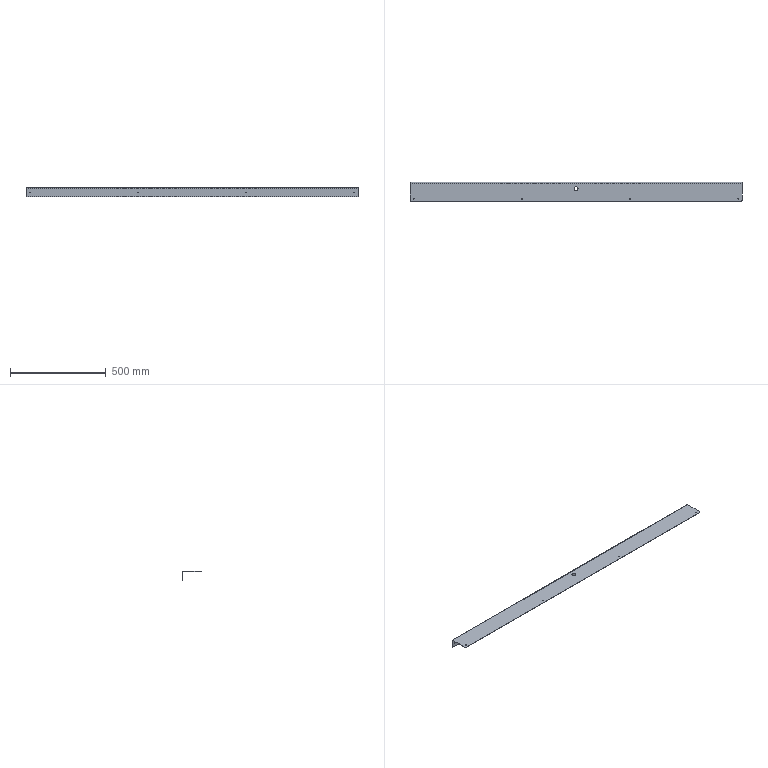Part | NX | features BREP 1 | 1 solid | 34 faces | box 1730 x 99.289 x 48.489 mm | volume 374057 mm3 | cylinder 22 | plane 12 | commonest cylinder face diameters 4.953 x16 12.7 x2 20.65 x2 6.35 x1 9.347 x1
STEP:
#1=CARTESIAN_POINT('',(1729.74,6.35,0.));
#2=VERTEX_POINT('',#1);
#3=CARTESIAN_POINT('',(1729.74,94.615,0.));
#4=VERTEX_POINT('',#3);
#5=CARTESIAN_POINT('',(1729.74,6.35,0.));
#6=DIRECTION('',(0.,1.,0.));
#7=VECTOR('',#6,1000.);
#8=LINE('',#5,#7);
#9=EDGE_CURVE('',#2,#4,#8,.T.);
#10=ORIENTED_EDGE('',*,*,#9,.T.);
#11=CARTESIAN_POINT('',(0.,94.615,0.));
#12=VERTEX_POINT('',#11);
#13=CARTESIAN_POINT('',(0.,94.615,0.));
#14=DIRECTION('',(1.,0.,0.));
#15=VECTOR('',#14,1000.);
#16=LINE('',#13,#15);
#17=EDGE_CURVE('',#12,#4,#16,.T.);
#18=ORIENTED_EDGE('',*,*,#17,.F.);
#19=CARTESIAN_POINT('',(0.,6.35,0.));
#20=VERTEX_POINT('',#19);
#21=CARTESIAN_POINT('',(0.,94.615,0.));
#22=DIRECTION('',(0.,-1.,0.));
#23=VECTOR('',#22,1000.);
#24=LINE('',#21,#23);
#25=EDGE_CURVE('',#12,#20,#24,.T.);
#26=ORIENTED_EDGE('',*,*,#25,.T.);
#27=CARTESIAN_POINT('',(6.35,0.,0.));
#28=VERTEX_POINT('',#27);
#29=CARTESIAN_POINT('',(6.35,6.35,0.));
#30=DIRECTION('',(0.,0.,1.));
#31=DIRECTION('',(-1.,0.,0.));
#32=AXIS2_PLACEMENT_3D('',#29,#30,#31);
#33=CIRCLE('',#32,6.35);
#34=EDGE_CURVE('',#20,#28,#33,.T.);
#35=ORIENTED_EDGE('',*,*,#34,.T.);
#36=CARTESIAN_POINT('',(1723.39,0.,0.));
#37=VERTEX_POINT('',#36);
#38=CARTESIAN_POINT('',(6.35,0.,0.));
#39=DIRECTION('',(1.,0.,0.));
#40=VECTOR('',#39,1000.);
#41=LINE('',#38,#40);
#42=EDGE_CURVE('',#28,#37,#41,.T.);
#43=ORIENTED_EDGE('',*,*,#42,.T.);
#44=CARTESIAN_POINT('',(1723.39,6.35,0.));
#45=DIRECTION('',(0.,0.,1.));
#46=DIRECTION('',(0.,-1.,0.));
#47=AXIS2_PLACEMENT_3D('',#44,#45,#46);
#48=CIRCLE('',#47,6.35);
#49=EDGE_CURVE('',#37,#2,#48,.T.);
#50=ORIENTED_EDGE('',*,*,#49,.T.);
#51=EDGE_LOOP('',(#10,#18,#26,#35,#43,#50));
#52=FACE_BOUND('',#51,.T.);
#53=CARTESIAN_POINT('',(21.526,15.24,0.));
#54=VERTEX_POINT('',#53);
#55=CARTESIAN_POINT('',(16.573,15.24,0.));
#56=VERTEX_POINT('',#55);
#57=CARTESIAN_POINT('',(19.05,15.24,0.));
#58=DIRECTION('',(0.,0.,1.));
#59=DIRECTION('',(1.,0.,0.));
#60=AXIS2_PLACEMENT_3D('',#57,#58,#59);
#61=CIRCLE('',#60,2.477);
#62=EDGE_CURVE('',#54,#56,#61,.T.);
#63=ORIENTED_EDGE('',*,*,#62,.F.);
#64=CARTESIAN_POINT('',(19.05,15.24,0.));
#65=DIRECTION('',(0.,0.,1.));
#66=DIRECTION('',(-1.,0.,0.));
#67=AXIS2_PLACEMENT_3D('',#64,#65,#66);
#68=CIRCLE('',#67,2.477);
#69=EDGE_CURVE('',#56,#54,#68,.T.);
#70=ORIENTED_EDGE('',*,*,#69,.F.);
#71=EDGE_LOOP('',(#63,#70));
#72=FACE_BOUND('',#71,.T.);
#73=CARTESIAN_POINT('',(585.407,15.24,0.));
#74=VERTEX_POINT('',#73);
#75=CARTESIAN_POINT('',(580.453,15.24,0.));
#76=VERTEX_POINT('',#75);
#77=CARTESIAN_POINT('',(582.93,15.24,0.));
#78=DIRECTION('',(0.,0.,1.));
#79=DIRECTION('',(1.,0.,0.));
#80=AXIS2_PLACEMENT_3D('',#77,#78,#79);
#81=CIRCLE('',#80,2.476);
#82=EDGE_CURVE('',#74,#76,#81,.T.);
#83=ORIENTED_EDGE('',*,*,#82,.F.);
#84=CARTESIAN_POINT('',(582.93,15.24,0.));
#85=DIRECTION('',(0.,0.,1.));
#86=DIRECTION('',(-1.,0.,0.));
#87=AXIS2_PLACEMENT_3D('',#84,#85,#86);
#88=CIRCLE('',#87,2.476);
#89=EDGE_CURVE('',#76,#74,#88,.T.);
#90=ORIENTED_EDGE('',*,*,#89,.F.);
#91=EDGE_LOOP('',(#83,#90));
#92=FACE_BOUND('',#91,.T.);
#93=CARTESIAN_POINT('',(1149.286,15.24,0.));
#94=VERTEX_POINT('',#93);
#95=CARTESIAN_POINT('',(1144.333,15.24,0.));
#96=VERTEX_POINT('',#95);
#97=CARTESIAN_POINT('',(1146.81,15.24,0.));
#98=DIRECTION('',(0.,0.,1.));
#99=DIRECTION('',(1.,0.,0.));
#100=AXIS2_PLACEMENT_3D('',#97,#98,#99);
#101=CIRCLE('',#100,2.476);
#102=EDGE_CURVE('',#94,#96,#101,.T.);
#103=ORIENTED_EDGE('',*,*,#102,.F.);
#104=CARTESIAN_POINT('',(1146.81,15.24,0.));
#105=DIRECTION('',(0.,0.,1.));
#106=DIRECTION('',(-1.,0.,0.));
#107=AXIS2_PLACEMENT_3D('',#104,#105,#106);
#108=CIRCLE('',#107,2.476);
#109=EDGE_CURVE('',#96,#94,#108,.T.);
#110=ORIENTED_EDGE('',*,*,#109,.F.);
#111=EDGE_LOOP('',(#103,#110));
#112=FACE_BOUND('',#111,.T.);
#113=CARTESIAN_POINT('',(1713.167,15.24,0.));
#114=VERTEX_POINT('',#113);
#115=CARTESIAN_POINT('',(1708.214,15.24,0.));
#116=VERTEX_POINT('',#115);
#117=CARTESIAN_POINT('',(1710.69,15.24,0.));
#118=DIRECTION('',(0.,0.,1.));
#119=DIRECTION('',(1.,0.,0.));
#120=AXIS2_PLACEMENT_3D('',#117,#118,#119);
#121=CIRCLE('',#120,2.476);
#122=EDGE_CURVE('',#114,#116,#121,.T.);
#123=ORIENTED_EDGE('',*,*,#122,.F.);
#124=CARTESIAN_POINT('',(1710.69,15.24,0.));
#125=DIRECTION('',(0.,0.,1.));
#126=DIRECTION('',(-1.,0.,0.));
#127=AXIS2_PLACEMENT_3D('',#124,#125,#126);
#128=CIRCLE('',#127,2.476);
#129=EDGE_CURVE('',#116,#114,#128,.T.);
#130=ORIENTED_EDGE('',*,*,#129,.F.);
#131=EDGE_LOOP('',(#123,#130));
#132=FACE_BOUND('',#131,.T.);
#133=CARTESIAN_POINT('',(875.322,66.802,0.));
#134=VERTEX_POINT('',#133);
#135=CARTESIAN_POINT('',(854.672,66.802,0.));
#136=VERTEX_POINT('',#135);
#137=CARTESIAN_POINT('',(864.997,66.802,0.));
#138=DIRECTION('',(0.,0.,1.));
#139=DIRECTION('',(1.,0.,0.));
#140=AXIS2_PLACEMENT_3D('',#137,#138,#139);
#141=CIRCLE('',#140,10.325);
#142=EDGE_CURVE('',#134,#136,#141,.T.);
#143=ORIENTED_EDGE('',*,*,#142,.F.);
#144=CARTESIAN_POINT('',(864.997,66.802,0.));
#145=DIRECTION('',(0.,0.,1.));
#146=DIRECTION('',(-1.,0.,0.));
#147=AXIS2_PLACEMENT_3D('',#144,#145,#146);
#148=CIRCLE('',#147,10.325);
#149=EDGE_CURVE('',#136,#134,#148,.T.);
#150=ORIENTED_EDGE('',*,*,#149,.F.);
#151=EDGE_LOOP('',(#143,#150));
#152=FACE_BOUND('',#151,.T.);
#153=CARTESIAN_POINT('',(0.,0.,0.));
#154=DIRECTION('',(0.,0.,1.));
#155=DIRECTION('',(1.,0.,0.));
#156=AXIS2_PLACEMENT_3D('',#153,#154,#155);
#157=PLANE('',#156);
#158=ADVANCED_FACE('',(#52,#72,#92,#112,#132,#152),#157,.T.);
#159=CARTESIAN_POINT('',(1729.74,6.35,-1.499));
#160=VERTEX_POINT('',#159);
#161=CARTESIAN_POINT('',(1723.39,0.,-1.499));
#162=VERTEX_POINT('',#161);
#163=CARTESIAN_POINT('',(1723.39,6.35,-1.499));
#164=DIRECTION('',(0.,0.,-1.));
#165=DIRECTION('',(1.,0.,0.));
#166=AXIS2_PLACEMENT_3D('',#163,#164,#165);
#167=CIRCLE('',#166,6.35);
#168=EDGE_CURVE('',#160,#162,#167,.T.);
#169=ORIENTED_EDGE('',*,*,#168,.F.);
#170=CARTESIAN_POINT('',(1729.74,6.35,-1.499));
#171=DIRECTION('',(0.,0.,1.));
#172=VECTOR('',#171,1000.);
#173=LINE('',#170,#172);
#174=EDGE_CURVE('',#160,#2,#173,.T.);
#175=ORIENTED_EDGE('',*,*,#174,.T.);
#176=ORIENTED_EDGE('',*,*,#49,.F.);
#177=CARTESIAN_POINT('',(1723.39,0.,-1.499));
#178=DIRECTION('',(0.,0.,1.));
#179=VECTOR('',#178,1000.);
#180=LINE('',#177,#179);
#181=EDGE_CURVE('',#162,#37,#180,.T.);
#182=ORIENTED_EDGE('',*,*,#181,.F.);
#183=EDGE_LOOP('',(#169,#175,#176,#182));
#184=FACE_BOUND('',#183,.T.);
#185=CARTESIAN_POINT('',(1723.39,6.35,-3.816));
#186=DIRECTION('',(0.,0.,1.));
#187=DIRECTION('',(0.,-1.,0.));
#188=AXIS2_PLACEMENT_3D('',#185,#186,#187);
#189=CYLINDRICAL_SURFACE('',#188,6.35);
#190=ADVANCED_FACE('',(#184),#189,.T.);
#191=ORIENTED_EDGE('',*,*,#42,.F.);
#192=CARTESIAN_POINT('',(6.35,0.,-1.499));
#193=VERTEX_POINT('',#192);
#194=CARTESIAN_POINT('',(6.35,0.,-1.499));
#195=DIRECTION('',(0.,0.,1.));
#196=VECTOR('',#195,1000.);
#197=LINE('',#194,#196);
#198=EDGE_CURVE('',#193,#28,#197,.T.);
#199=ORIENTED_EDGE('',*,*,#198,.F.);
#200=CARTESIAN_POINT('',(6.35,0.,-1.499));
#201=DIRECTION('',(1.,0.,0.));
#202=VECTOR('',#201,1000.);
#203=LINE('',#200,#202);
#204=EDGE_CURVE('',#193,#162,#203,.T.);
#205=ORIENTED_EDGE('',*,*,#204,.T.);
#206=ORIENTED_EDGE('',*,*,#181,.T.);
#207=EDGE_LOOP('',(#191,#199,#205,#206));
#208=FACE_BOUND('',#207,.T.);
#209=CARTESIAN_POINT('',(864.87,0.,-0.7493));
#210=DIRECTION('',(0.,-1.,0.));
#211=DIRECTION('',(0.,0.,-1.));
#212=AXIS2_PLACEMENT_3D('',#209,#210,#211);
#213=PLANE('',#212);
#214=ADVANCED_FACE('',(#208),#213,.T.);
#215=ORIENTED_EDGE('',*,*,#204,.F.);
#216=CARTESIAN_POINT('',(0.,6.35,-1.499));
#217=VERTEX_POINT('',#216);
#218=CARTESIAN_POINT('',(6.35,6.35,-1.499));
#219=DIRECTION('',(0.,0.,-1.));
#220=DIRECTION('',(0.,-1.,0.));
#221=AXIS2_PLACEMENT_3D('',#218,#219,#220);
#222=CIRCLE('',#221,6.35);
#223=EDGE_CURVE('',#193,#217,#222,.T.);
#224=ORIENTED_EDGE('',*,*,#223,.T.);
#225=CARTESIAN_POINT('',(0.,94.615,-1.499));
#226=VERTEX_POINT('',#225);
#227=CARTESIAN_POINT('',(0.,94.615,-1.499));
#228=DIRECTION('',(0.,-1.,0.));
#229=VECTOR('',#228,1000.);
#230=LINE('',#227,#229);
#231=EDGE_CURVE('',#226,#217,#230,.T.);
#232=ORIENTED_EDGE('',*,*,#231,.F.);
#233=CARTESIAN_POINT('',(1729.74,94.615,-1.499));
#234=VERTEX_POINT('',#233);
#235=CARTESIAN_POINT('',(0.,94.615,-1.499));
#236=DIRECTION('',(1.,0.,0.));
#237=VECTOR('',#236,1000.);
#238=LINE('',#235,#237);
#239=EDGE_CURVE('',#226,#234,#238,.T.);
#240=ORIENTED_EDGE('',*,*,#239,.T.);
#241=CARTESIAN_POINT('',(1729.74,6.35,-1.499));
#242=DIRECTION('',(0.,1.,0.));
#243=VECTOR('',#242,1000.);
#244=LINE('',#241,#243);
#245=EDGE_CURVE('',#160,#234,#244,.T.);
#246=ORIENTED_EDGE('',*,*,#245,.F.);
#247=ORIENTED_EDGE('',*,*,#168,.T.);
#248=EDGE_LOOP('',(#215,#224,#232,#240,#246,#247));
#249=FACE_BOUND('',#248,.T.);
#250=CARTESIAN_POINT('',(21.526,15.24,-1.499));
#251=VERTEX_POINT('',#250);
#252=CARTESIAN_POINT('',(16.573,15.24,-1.499));
#253=VERTEX_POINT('',#252);
#254=CARTESIAN_POINT('',(19.05,15.24,-1.499));
#255=DIRECTION('',(0.,0.,1.));
#256=DIRECTION('',(1.,0.,0.));
#257=AXIS2_PLACEMENT_3D('',#254,#255,#256);
#258=CIRCLE('',#257,2.477);
#259=EDGE_CURVE('',#251,#253,#258,.T.);
#260=ORIENTED_EDGE('',*,*,#259,.T.);
#261=CARTESIAN_POINT('',(19.05,15.24,-1.499));
#262=DIRECTION('',(0.,0.,1.));
#263=DIRECTION('',(-1.,0.,0.));
#264=AXIS2_PLACEMENT_3D('',#261,#262,#263);
#265=CIRCLE('',#264,2.477);
#266=EDGE_CURVE('',#253,#251,#265,.T.);
#267=ORIENTED_EDGE('',*,*,#266,.T.);
#268=EDGE_LOOP('',(#260,#267));
#269=FACE_BOUND('',#268,.T.);
#270=CARTESIAN_POINT('',(585.407,15.24,-1.499));
#271=VERTEX_POINT('',#270);
#272=CARTESIAN_POINT('',(580.453,15.24,-1.499));
#273=VERTEX_POINT('',#272);
#274=CARTESIAN_POINT('',(582.93,15.24,-1.499));
#275=DIRECTION('',(0.,0.,1.));
#276=DIRECTION('',(1.,0.,0.));
#277=AXIS2_PLACEMENT_3D('',#274,#275,#276);
#278=CIRCLE('',#277,2.476);
#279=EDGE_CURVE('',#271,#273,#278,.T.);
#280=ORIENTED_EDGE('',*,*,#279,.T.);
#281=CARTESIAN_POINT('',(582.93,15.24,-1.499));
#282=DIRECTION('',(0.,0.,1.));
#283=DIRECTION('',(-1.,0.,0.));
#284=AXIS2_PLACEMENT_3D('',#281,#282,#283);
#285=CIRCLE('',#284,2.476);
#286=EDGE_CURVE('',#273,#271,#285,.T.);
#287=ORIENTED_EDGE('',*,*,#286,.T.);
#288=EDGE_LOOP('',(#280,#287));
#289=FACE_BOUND('',#288,.T.);
#290=CARTESIAN_POINT('',(1149.286,15.24,-1.499));
#291=VERTEX_POINT('',#290);
#292=CARTESIAN_POINT('',(1144.333,15.24,-1.499));
#293=VERTEX_POINT('',#292);
#294=CARTESIAN_POINT('',(1146.81,15.24,-1.499));
#295=DIRECTION('',(0.,0.,1.));
#296=DIRECTION('',(1.,0.,0.));
#297=AXIS2_PLACEMENT_3D('',#294,#295,#296);
#298=CIRCLE('',#297,2.476);
#299=EDGE_CURVE('',#291,#293,#298,.T.);
#300=ORIENTED_EDGE('',*,*,#299,.T.);
#301=CARTESIAN_POINT('',(1146.81,15.24,-1.499));
#302=DIRECTION('',(0.,0.,1.));
#303=DIRECTION('',(-1.,0.,0.));
#304=AXIS2_PLACEMENT_3D('',#301,#302,#303);
#305=CIRCLE('',#304,2.476);
#306=EDGE_CURVE('',#293,#291,#305,.T.);
#307=ORIENTED_EDGE('',*,*,#306,.T.);
#308=EDGE_LOOP('',(#300,#307));
#309=FACE_BOUND('',#308,.T.);
#310=CARTESIAN_POINT('',(1713.167,15.24,-1.499));
#311=VERTEX_POINT('',#310);
#312=CARTESIAN_POINT('',(1708.214,15.24,-1.499));
#313=VERTEX_POINT('',#312);
#314=CARTESIAN_POINT('',(1710.69,15.24,-1.499));
#315=DIRECTION('',(0.,0.,1.));
#316=DIRECTION('',(1.,0.,0.));
#317=AXIS2_PLACEMENT_3D('',#314,#315,#316);
#318=CIRCLE('',#317,2.476);
#319=EDGE_CURVE('',#311,#313,#318,.T.);
#320=ORIENTED_EDGE('',*,*,#319,.T.);
#321=CARTESIAN_POINT('',(1710.69,15.24,-1.499));
#322=DIRECTION('',(0.,0.,1.));
#323=DIRECTION('',(-1.,0.,0.));
#324=AXIS2_PLACEMENT_3D('',#321,#322,#323);
#325=CIRCLE('',#324,2.476);
#326=EDGE_CURVE('',#313,#311,#325,.T.);
#327=ORIENTED_EDGE('',*,*,#326,.T.);
#328=EDGE_LOOP('',(#320,#327));
#329=FACE_BOUND('',#328,.T.);
#330=CARTESIAN_POINT('',(875.322,66.802,-1.499));
#331=VERTEX_POINT('',#330);
#332=CARTESIAN_POINT('',(854.672,66.802,-1.499));
#333=VERTEX_POINT('',#332);
#334=CARTESIAN_POINT('',(864.997,66.802,-1.499));
#335=DIRECTION('',(0.,0.,1.));
#336=DIRECTION('',(1.,0.,0.));
#337=AXIS2_PLACEMENT_3D('',#334,#335,#336);
#338=CIRCLE('',#337,10.325);
#339=EDGE_CURVE('',#331,#333,#338,.T.);
#340=ORIENTED_EDGE('',*,*,#339,.T.);
#341=CARTESIAN_POINT('',(864.997,66.802,-1.499));
#342=DIRECTION('',(0.,0.,1.));
#343=DIRECTION('',(-1.,0.,0.));
#344=AXIS2_PLACEMENT_3D('',#341,#342,#343);
#345=CIRCLE('',#344,10.325);
#346=EDGE_CURVE('',#333,#331,#345,.T.);
#347=ORIENTED_EDGE('',*,*,#346,.T.);
#348=EDGE_LOOP('',(#340,#347));
#349=FACE_BOUND('',#348,.T.);
#350=CARTESIAN_POINT('',(0.,0.,-1.499));
#351=DIRECTION('',(0.,0.,1.));
#352=DIRECTION('',(1.,0.,0.));
#353=AXIS2_PLACEMENT_3D('',#350,#351,#352);
#354=PLANE('',#353);
#355=ADVANCED_FACE('',(#249,#269,#289,#309,#329,#349),#354,.F.);
#356=ORIENTED_EDGE('',*,*,#245,.T.);
#357=CARTESIAN_POINT('',(1729.74,94.615,-1.499));
#358=DIRECTION('',(0.,0.,1.));
#359=VECTOR('',#358,1000.);
#360=LINE('',#357,#359);
#361=EDGE_CURVE('',#234,#4,#360,.T.);
#362=ORIENTED_EDGE('',*,*,#361,.T.);
#363=ORIENTED_EDGE('',*,*,#9,.F.);
#364=ORIENTED_EDGE('',*,*,#174,.F.);
#365=EDGE_LOOP('',(#356,#362,#363,#364));
#366=FACE_BOUND('',#365,.T.);
#367=CARTESIAN_POINT('',(1729.74,48.895,-0.7493));
#368=DIRECTION('',(1.,0.,0.));
#369=DIRECTION('',(0.,1.,0.));
#370=AXIS2_PLACEMENT_3D('',#367,#368,#369);
#371=PLANE('',#370);
#372=ADVANCED_FACE('',(#366),#371,.T.);
#373=CARTESIAN_POINT('',(1729.74,97.79,-4.674));
#374=VERTEX_POINT('',#373);
#375=CARTESIAN_POINT('',(1729.74,99.289,-4.674));
#376=VERTEX_POINT('',#375);
#377=CARTESIAN_POINT('',(1729.74,97.79,-4.674));
#378=DIRECTION('',(0.,1.,0.));
#379=VECTOR('',#378,1000.);
#380=LINE('',#377,#379);
#381=EDGE_CURVE('',#374,#376,#380,.T.);
#382=ORIENTED_EDGE('',*,*,#381,.T.);
#383=CARTESIAN_POINT('',(1729.74,94.615,-4.674));
#384=DIRECTION('',(1.,0.,0.));
#385=DIRECTION('',(0.,1.,0.));
#386=AXIS2_PLACEMENT_3D('',#383,#384,#385);
#387=CIRCLE('',#386,4.674);
#388=EDGE_CURVE('',#376,#4,#387,.T.);
#389=ORIENTED_EDGE('',*,*,#388,.T.);
#390=ORIENTED_EDGE('',*,*,#361,.F.);
#391=CARTESIAN_POINT('',(1729.74,94.615,-4.674));
#392=DIRECTION('',(1.,0.,0.));
#393=DIRECTION('',(0.,1.,0.));
#394=AXIS2_PLACEMENT_3D('',#391,#392,#393);
#395=CIRCLE('',#394,3.175);
#396=EDGE_CURVE('',#374,#234,#395,.T.);
#397=ORIENTED_EDGE('',*,*,#396,.F.);
#398=EDGE_LOOP('',(#382,#389,#390,#397));
#399=FACE_BOUND('',#398,.T.);
#400=CARTESIAN_POINT('',(1729.74,97.39,-1.899));
#401=DIRECTION('',(1.,0.,0.));
#402=DIRECTION('',(0.,1.,0.));
#403=AXIS2_PLACEMENT_3D('',#400,#401,#402);
#404=PLANE('',#403);
#405=ADVANCED_FACE('',(#399),#404,.T.);
#406=ORIENTED_EDGE('',*,*,#396,.T.);
#407=ORIENTED_EDGE('',*,*,#239,.F.);
#408=CARTESIAN_POINT('',(0.,97.79,-4.674));
#409=VERTEX_POINT('',#408);
#410=CARTESIAN_POINT('',(0.,94.615,-4.674));
#411=DIRECTION('',(1.,0.,0.));
#412=DIRECTION('',(0.,1.,0.));
#413=AXIS2_PLACEMENT_3D('',#410,#411,#412);
#414=CIRCLE('',#413,3.175);
#415=EDGE_CURVE('',#409,#226,#414,.T.);
#416=ORIENTED_EDGE('',*,*,#415,.F.);
#417=CARTESIAN_POINT('',(0.,97.79,-4.674));
#418=DIRECTION('',(1.,0.,0.));
#419=VECTOR('',#418,1000.);
#420=LINE('',#417,#419);
#421=EDGE_CURVE('',#409,#374,#420,.T.);
#422=ORIENTED_EDGE('',*,*,#421,.T.);
#423=EDGE_LOOP('',(#406,#407,#416,#422));
#424=FACE_BOUND('',#423,.T.);
#425=CARTESIAN_POINT('',(0.,94.615,-4.674));
#426=DIRECTION('',(1.,0.,0.));
#427=DIRECTION('',(0.,1.,0.));
#428=AXIS2_PLACEMENT_3D('',#425,#426,#427);
#429=CYLINDRICAL_SURFACE('',#428,3.175);
#430=ADVANCED_FACE('',(#424),#429,.F.);
#431=ORIENTED_EDGE('',*,*,#421,.F.);
#432=CARTESIAN_POINT('',(0.,97.79,-48.489));
#433=VERTEX_POINT('',#432);
#434=CARTESIAN_POINT('',(0.,97.79,-48.489));
#435=DIRECTION('',(0.,0.,1.));
#436=VECTOR('',#435,1000.);
#437=LINE('',#434,#436);
#438=EDGE_CURVE('',#433,#409,#437,.T.);
#439=ORIENTED_EDGE('',*,*,#438,.F.);
#440=CARTESIAN_POINT('',(1729.74,97.79,-48.489));
#441=VERTEX_POINT('',#440);
#442=CARTESIAN_POINT('',(1729.74,97.79,-48.489));
#443=DIRECTION('',(-1.,0.,0.));
#444=VECTOR('',#443,1000.);
#445=LINE('',#442,#444);
#446=EDGE_CURVE('',#441,#433,#445,.T.);
#447=ORIENTED_EDGE('',*,*,#446,.F.);
#448=CARTESIAN_POINT('',(1729.74,97.79,-4.674));
#449=DIRECTION('',(0.,0.,-1.));
#450=VECTOR('',#449,1000.);
#451=LINE('',#448,#450);
#452=EDGE_CURVE('',#374,#441,#451,.T.);
#453=ORIENTED_EDGE('',*,*,#452,.F.);
#454=EDGE_LOOP('',(#431,#439,#447,#453));
#455=FACE_BOUND('',#454,.T.);
#456=CARTESIAN_POINT('',(21.526,97.79,-26.899));
#457=VERTEX_POINT('',#456);
#458=CARTESIAN_POINT('',(16.573,97.79,-26.899));
#459=VERTEX_POINT('',#458);
#460=CARTESIAN_POINT('',(19.05,97.79,-26.899));
#461=DIRECTION('',(0.,1.,0.));
#462=DIRECTION('',(1.,0.,0.));
#463=AXIS2_PLACEMENT_3D('',#460,#461,#462);
#464=CIRCLE('',#463,2.477);
#465=EDGE_CURVE('',#457,#459,#464,.T.);
#466=ORIENTED_EDGE('',*,*,#465,.T.);
#467=CARTESIAN_POINT('',(19.05,97.79,-26.899));
#468=DIRECTION('',(0.,1.,0.));
#469=DIRECTION('',(-1.,0.,0.));
#470=AXIS2_PLACEMENT_3D('',#467,#468,#469);
#471=CIRCLE('',#470,2.477);
#472=EDGE_CURVE('',#459,#457,#471,.T.);
#473=ORIENTED_EDGE('',*,*,#472,.T.);
#474=EDGE_LOOP('',(#466,#473));
#475=FACE_BOUND('',#474,.T.);
#476=CARTESIAN_POINT('',(585.407,97.79,-26.899));
#477=VERTEX_POINT('',#476);
#478=CARTESIAN_POINT('',(580.453,97.79,-26.899));
#479=VERTEX_POINT('',#478);
#480=CARTESIAN_POINT('',(582.93,97.79,-26.899));
#481=DIRECTION('',(0.,1.,0.));
#482=DIRECTION('',(1.,0.,0.));
#483=AXIS2_PLACEMENT_3D('',#480,#481,#482);
#484=CIRCLE('',#483,2.476);
#485=EDGE_CURVE('',#477,#479,#484,.T.);
#486=ORIENTED_EDGE('',*,*,#485,.T.);
#487=CARTESIAN_POINT('',(582.93,97.79,-26.899));
#488=DIRECTION('',(0.,1.,0.));
#489=DIRECTION('',(-1.,0.,0.));
#490=AXIS2_PLACEMENT_3D('',#487,#488,#489);
#491=CIRCLE('',#490,2.476);
#492=EDGE_CURVE('',#479,#477,#491,.T.);
#493=ORIENTED_EDGE('',*,*,#492,.T.);
#494=EDGE_LOOP('',(#486,#493));
#495=FACE_BOUND('',#494,.T.);
#496=CARTESIAN_POINT('',(1149.286,97.79,-26.899));
#497=VERTEX_POINT('',#496);
#498=CARTESIAN_POINT('',(1144.333,97.79,-26.899));
#499=VERTEX_POINT('',#498);
#500=CARTESIAN_POINT('',(1146.81,97.79,-26.899));
#501=DIRECTION('',(0.,1.,0.));
#502=DIRECTION('',(1.,0.,0.));
#503=AXIS2_PLACEMENT_3D('',#500,#501,#502);
#504=CIRCLE('',#503,2.476);
#505=EDGE_CURVE('',#497,#499,#504,.T.);
#506=ORIENTED_EDGE('',*,*,#505,.T.);
#507=CARTESIAN_POINT('',(1146.81,97.79,-26.899));
#508=DIRECTION('',(0.,1.,0.));
#509=DIRECTION('',(-1.,0.,0.));
#510=AXIS2_PLACEMENT_3D('',#507,#508,#509);
#511=CIRCLE('',#510,2.476);
#512=EDGE_CURVE('',#499,#497,#511,.T.);
#513=ORIENTED_EDGE('',*,*,#512,.T.);
#514=EDGE_LOOP('',(#506,#513));
#515=FACE_BOUND('',#514,.T.);
#516=CARTESIAN_POINT('',(1713.167,97.79,-26.899));
#517=VERTEX_POINT('',#516);
#518=CARTESIAN_POINT('',(1708.214,97.79,-26.899));
#519=VERTEX_POINT('',#518);
#520=CARTESIAN_POINT('',(1710.69,97.79,-26.899));
#521=DIRECTION('',(0.,1.,0.));
#522=DIRECTION('',(1.,0.,0.));
#523=AXIS2_PLACEMENT_3D('',#520,#521,#522);
#524=CIRCLE('',#523,2.476);
#525=EDGE_CURVE('',#517,#519,#524,.T.);
#526=ORIENTED_EDGE('',*,*,#525,.T.);
#527=CARTESIAN_POINT('',(1710.69,97.79,-26.899));
#528=DIRECTION('',(0.,1.,0.));
#529=DIRECTION('',(-1.,0.,0.));
#530=AXIS2_PLACEMENT_3D('',#527,#528,#529);
#531=CIRCLE('',#530,2.476);
#532=EDGE_CURVE('',#519,#517,#531,.T.);
#533=ORIENTED_EDGE('',*,*,#532,.T.);
#534=EDGE_LOOP('',(#526,#533));
#535=FACE_BOUND('',#534,.T.);
#536=CARTESIAN_POINT('',(1318.754,97.79,-1.499));
#537=DIRECTION('',(0.,1.,0.));
#538=DIRECTION('',(1.,0.,0.));
#539=AXIS2_PLACEMENT_3D('',#536,#537,#538);
#540=PLANE('',#539);
#541=ADVANCED_FACE('',(#455,#475,#495,#515,#535),#540,.F.);
#542=CARTESIAN_POINT('',(1729.74,99.289,-48.489));
#543=VERTEX_POINT('',#542);
#544=CARTESIAN_POINT('',(1729.74,97.79,-48.489));
#545=DIRECTION('',(0.,1.,0.));
#546=VECTOR('',#545,1000.);
#547=LINE('',#544,#546);
#548=EDGE_CURVE('',#441,#543,#547,.T.);
#549=ORIENTED_EDGE('',*,*,#548,.T.);
#550=CARTESIAN_POINT('',(1729.74,99.289,-4.674));
#551=DIRECTION('',(0.,0.,-1.));
#552=VECTOR('',#551,1000.);
#553=LINE('',#550,#552);
#554=EDGE_CURVE('',#376,#543,#553,.T.);
#555=ORIENTED_EDGE('',*,*,#554,.F.);
#556=ORIENTED_EDGE('',*,*,#381,.F.);
#557=ORIENTED_EDGE('',*,*,#452,.T.);
#558=EDGE_LOOP('',(#549,#555,#556,#557));
#559=FACE_BOUND('',#558,.T.);
#560=CARTESIAN_POINT('',(1729.74,98.539,-26.581));
#561=DIRECTION('',(-1.,0.,0.));
#562=DIRECTION('',(0.,0.,1.));
#563=AXIS2_PLACEMENT_3D('',#560,#561,#562);
#564=PLANE('',#563);
#565=ADVANCED_FACE('',(#559),#564,.F.);
#566=CARTESIAN_POINT('',(0.,99.289,-48.489));
#567=VERTEX_POINT('',#566);
#568=CARTESIAN_POINT('',(1729.74,99.289,-48.489));
#569=DIRECTION('',(-1.,0.,0.));
#570=VECTOR('',#569,1000.);
#571=LINE('',#568,#570);
#572=EDGE_CURVE('',#543,#567,#571,.T.);
#573=ORIENTED_EDGE('',*,*,#572,.T.);
#574=CARTESIAN_POINT('',(0.,99.289,-4.674));
#575=VERTEX_POINT('',#574);
#576=CARTESIAN_POINT('',(0.,99.289,-48.489));
#577=DIRECTION('',(0.,0.,1.));
#578=VECTOR('',#577,1000.);
#579=LINE('',#576,#578);
#580=EDGE_CURVE('',#567,#575,#579,.T.);
#581=ORIENTED_EDGE('',*,*,#580,.T.);
#582=CARTESIAN_POINT('',(0.,99.289,-4.674));
#583=DIRECTION('',(1.,0.,0.));
#584=VECTOR('',#583,1000.);
#585=LINE('',#582,#584);
#586=EDGE_CURVE('',#575,#376,#585,.T.);
#587=ORIENTED_EDGE('',*,*,#586,.T.);
#588=ORIENTED_EDGE('',*,*,#554,.T.);
#589=EDGE_LOOP('',(#573,#581,#587,#588));
#590=FACE_BOUND('',#589,.T.);
#591=CARTESIAN_POINT('',(21.526,99.289,-26.899));
#592=VERTEX_POINT('',#591);
#593=CARTESIAN_POINT('',(16.573,99.289,-26.899));
#594=VERTEX_POINT('',#593);
#595=CARTESIAN_POINT('',(19.05,99.289,-26.899));
#596=DIRECTION('',(0.,1.,0.));
#597=DIRECTION('',(1.,0.,0.));
#598=AXIS2_PLACEMENT_3D('',#595,#596,#597);
#599=CIRCLE('',#598,2.477);
#600=EDGE_CURVE('',#592,#594,#599,.T.);
#601=ORIENTED_EDGE('',*,*,#600,.F.);
#602=CARTESIAN_POINT('',(19.05,99.289,-26.899));
#603=DIRECTION('',(0.,1.,0.));
#604=DIRECTION('',(-1.,0.,0.));
#605=AXIS2_PLACEMENT_3D('',#602,#603,#604);
#606=CIRCLE('',#605,2.477);
#607=EDGE_CURVE('',#594,#592,#606,.T.);
#608=ORIENTED_EDGE('',*,*,#607,.F.);
#609=EDGE_LOOP('',(#601,#608));
#610=FACE_BOUND('',#609,.T.);
#611=CARTESIAN_POINT('',(585.407,99.289,-26.899));
#612=VERTEX_POINT('',#611);
#613=CARTESIAN_POINT('',(580.453,99.289,-26.899));
#614=VERTEX_POINT('',#613);
#615=CARTESIAN_POINT('',(582.93,99.289,-26.899));
#616=DIRECTION('',(0.,1.,0.));
#617=DIRECTION('',(1.,0.,0.));
#618=AXIS2_PLACEMENT_3D('',#615,#616,#617);
#619=CIRCLE('',#618,2.476);
#620=EDGE_CURVE('',#612,#614,#619,.T.);
#621=ORIENTED_EDGE('',*,*,#620,.F.);
#622=CARTESIAN_POINT('',(582.93,99.289,-26.899));
#623=DIRECTION('',(0.,1.,0.));
#624=DIRECTION('',(-1.,0.,0.));
#625=AXIS2_PLACEMENT_3D('',#622,#623,#624);
#626=CIRCLE('',#625,2.476);
#627=EDGE_CURVE('',#614,#612,#626,.T.);
#628=ORIENTED_EDGE('',*,*,#627,.F.);
#629=EDGE_LOOP('',(#621,#628));
#630=FACE_BOUND('',#629,.T.);
#631=CARTESIAN_POINT('',(1149.286,99.289,-26.899));
#632=VERTEX_POINT('',#631);
#633=CARTESIAN_POINT('',(1144.333,99.289,-26.899));
#634=VERTEX_POINT('',#633);
#635=CARTESIAN_POINT('',(1146.81,99.289,-26.899));
#636=DIRECTION('',(0.,1.,0.));
#637=DIRECTION('',(1.,0.,0.));
#638=AXIS2_PLACEMENT_3D('',#635,#636,#637);
#639=CIRCLE('',#638,2.476);
#640=EDGE_CURVE('',#632,#634,#639,.T.);
#641=ORIENTED_EDGE('',*,*,#640,.F.);
#642=CARTESIAN_POINT('',(1146.81,99.289,-26.899));
#643=DIRECTION('',(0.,1.,0.));
#644=DIRECTION('',(-1.,0.,0.));
#645=AXIS2_PLACEMENT_3D('',#642,#643,#644);
#646=CIRCLE('',#645,2.476);
#647=EDGE_CURVE('',#634,#632,#646,.T.);
#648=ORIENTED_EDGE('',*,*,#647,.F.);
#649=EDGE_LOOP('',(#641,#648));
#650=FACE_BOUND('',#649,.T.);
#651=CARTESIAN_POINT('',(1713.167,99.289,-26.899));
#652=VERTEX_POINT('',#651);
#653=CARTESIAN_POINT('',(1708.214,99.289,-26.899));
#654=VERTEX_POINT('',#653);
#655=CARTESIAN_POINT('',(1710.69,99.289,-26.899));
#656=DIRECTION('',(0.,1.,0.));
#657=DIRECTION('',(1.,0.,0.));
#658=AXIS2_PLACEMENT_3D('',#655,#656,#657);
#659=CIRCLE('',#658,2.476);
#660=EDGE_CURVE('',#652,#654,#659,.T.);
#661=ORIENTED_EDGE('',*,*,#660,.F.);
#662=CARTESIAN_POINT('',(1710.69,99.289,-26.899));
#663=DIRECTION('',(0.,1.,0.));
#664=DIRECTION('',(-1.,0.,0.));
#665=AXIS2_PLACEMENT_3D('',#662,#663,#664);
#666=CIRCLE('',#665,2.476);
#667=EDGE_CURVE('',#654,#652,#666,.T.);
#668=ORIENTED_EDGE('',*,*,#667,.F.);
#669=EDGE_LOOP('',(#661,#668));
#670=FACE_BOUND('',#669,.T.);
#671=CARTESIAN_POINT('',(1318.754,99.289,-1.499));
#672=DIRECTION('',(0.,1.,0.));
#673=DIRECTION('',(1.,0.,0.));
#674=AXIS2_PLACEMENT_3D('',#671,#672,#673);
#675=PLANE('',#674);
#676=ADVANCED_FACE('',(#590,#610,#630,#650,#670),#675,.T.);
#677=CARTESIAN_POINT('',(0.,94.615,-4.674));
#678=DIRECTION('',(1.,0.,0.));
#679=DIRECTION('',(0.,1.,0.));
#680=AXIS2_PLACEMENT_3D('',#677,#678,#679);
#681=CIRCLE('',#680,4.674);
#682=EDGE_CURVE('',#575,#12,#681,.T.);
#683=ORIENTED_EDGE('',*,*,#682,.T.);
#684=ORIENTED_EDGE('',*,*,#17,.T.);
#685=ORIENTED_EDGE('',*,*,#388,.F.);
#686=ORIENTED_EDGE('',*,*,#586,.F.);
#687=EDGE_LOOP('',(#683,#684,#685,#686));
#688=FACE_BOUND('',#687,.T.);
#689=CARTESIAN_POINT('',(0.,94.615,-4.674));
#690=DIRECTION('',(1.,0.,0.));
#691=DIRECTION('',(0.,1.,0.));
#692=AXIS2_PLACEMENT_3D('',#689,#690,#691);
#693=CYLINDRICAL_SURFACE('',#692,4.674);
#694=ADVANCED_FACE('',(#688),#693,.T.);
#695=CARTESIAN_POINT('',(0.,94.615,-1.499));
#696=DIRECTION('',(0.,0.,1.));
#697=VECTOR('',#696,1000.);
#698=LINE('',#695,#697);
#699=EDGE_CURVE('',#226,#12,#698,.T.);
#700=ORIENTED_EDGE('',*,*,#699,.T.);
#701=ORIENTED_EDGE('',*,*,#682,.F.);
#702=CARTESIAN_POINT('',(0.,97.79,-4.674));
#703=DIRECTION('',(0.,1.,0.));
#704=VECTOR('',#703,1000.);
#705=LINE('',#702,#704);
#706=EDGE_CURVE('',#409,#575,#705,.T.);
#707=ORIENTED_EDGE('',*,*,#706,.F.);
#708=ORIENTED_EDGE('',*,*,#415,.T.);
#709=EDGE_LOOP('',(#700,#701,#707,#708));
#710=FACE_BOUND('',#709,.T.);
#711=CARTESIAN_POINT('',(0.,97.39,-1.899));
#712=DIRECTION('',(1.,0.,0.));
#713=DIRECTION('',(0.,1.,0.));
#714=AXIS2_PLACEMENT_3D('',#711,#712,#713);
#715=PLANE('',#714);
#716=ADVANCED_FACE('',(#710),#715,.F.);
#717=ORIENTED_EDGE('',*,*,#706,.T.);
#718=ORIENTED_EDGE('',*,*,#580,.F.);
#719=CARTESIAN_POINT('',(0.,97.79,-48.489));
#720=DIRECTION('',(0.,1.,0.));
#721=VECTOR('',#720,1000.);
#722=LINE('',#719,#721);
#723=EDGE_CURVE('',#433,#567,#722,.T.);
#724=ORIENTED_EDGE('',*,*,#723,.F.);
#725=ORIENTED_EDGE('',*,*,#438,.T.);
#726=EDGE_LOOP('',(#717,#718,#724,#725));
#727=FACE_BOUND('',#726,.T.);
#728=CARTESIAN_POINT('',(0.,98.539,-26.581));
#729=DIRECTION('',(1.,0.,0.));
#730=DIRECTION('',(0.,1.,0.));
#731=AXIS2_PLACEMENT_3D('',#728,#729,#730);
#732=PLANE('',#731);
#733=ADVANCED_FACE('',(#727),#732,.F.);
#734=ORIENTED_EDGE('',*,*,#723,.T.);
#735=ORIENTED_EDGE('',*,*,#572,.F.);
#736=ORIENTED_EDGE('',*,*,#548,.F.);
#737=ORIENTED_EDGE('',*,*,#446,.T.);
#738=EDGE_LOOP('',(#734,#735,#736,#737));
#739=FACE_BOUND('',#738,.T.);
#740=CARTESIAN_POINT('',(864.87,98.539,-48.489));
#741=DIRECTION('',(0.,0.,1.));
#742=DIRECTION('',(1.,0.,0.));
#743=AXIS2_PLACEMENT_3D('',#740,#741,#742);
#744=PLANE('',#743);
#745=ADVANCED_FACE('',(#739),#744,.F.);
#746=ORIENTED_EDGE('',*,*,#25,.F.);
#747=ORIENTED_EDGE('',*,*,#699,.F.);
#748=ORIENTED_EDGE('',*,*,#231,.T.);
#749=CARTESIAN_POINT('',(0.,6.35,-1.499));
#750=DIRECTION('',(0.,0.,1.));
#751=VECTOR('',#750,1000.);
#752=LINE('',#749,#751);
#753=EDGE_CURVE('',#217,#20,#752,.T.);
#754=ORIENTED_EDGE('',*,*,#753,.T.);
#755=EDGE_LOOP('',(#746,#747,#748,#754));
#756=FACE_BOUND('',#755,.T.);
#757=CARTESIAN_POINT('',(0.,48.895,-0.7493));
#758=DIRECTION('',(-1.,0.,0.));
#759=DIRECTION('',(0.,0.,1.));
#760=AXIS2_PLACEMENT_3D('',#757,#758,#759);
#761=PLANE('',#760);
#762=ADVANCED_FACE('',(#756),#761,.T.);
#763=ORIENTED_EDGE('',*,*,#223,.F.);
#764=ORIENTED_EDGE('',*,*,#198,.T.);
#765=ORIENTED_EDGE('',*,*,#34,.F.);
#766=ORIENTED_EDGE('',*,*,#753,.F.);
#767=EDGE_LOOP('',(#763,#764,#765,#766));
#768=FACE_BOUND('',#767,.T.);
#769=CARTESIAN_POINT('',(6.35,6.35,-3.816));
#770=DIRECTION('',(0.,0.,1.));
#771=DIRECTION('',(-1.,0.,0.));
#772=AXIS2_PLACEMENT_3D('',#769,#770,#771);
#773=CYLINDRICAL_SURFACE('',#772,6.35);
#774=ADVANCED_FACE('',(#768),#773,.T.);
#775=CARTESIAN_POINT('',(21.526,99.289,-26.899));
#776=DIRECTION('',(0.,-1.,0.));
#777=VECTOR('',#776,1000.);
#778=LINE('',#775,#777);
#779=EDGE_CURVE('',#457,#592,#778,.F.);
#780=ORIENTED_EDGE('',*,*,#779,.F.);
#781=ORIENTED_EDGE('',*,*,#472,.F.);
#782=CARTESIAN_POINT('',(16.573,99.289,-26.899));
#783=DIRECTION('',(0.,-1.,0.));
#784=VECTOR('',#783,1000.);
#785=LINE('',#782,#784);
#786=EDGE_CURVE('',#459,#594,#785,.F.);
#787=ORIENTED_EDGE('',*,*,#786,.T.);
#788=ORIENTED_EDGE('',*,*,#607,.T.);
#789=EDGE_LOOP('',(#780,#781,#787,#788));
#790=FACE_BOUND('',#789,.T.);
#791=CARTESIAN_POINT('',(19.05,98.539,-26.899));
#792=DIRECTION('',(0.,1.,0.));
#793=DIRECTION('',(-1.,0.,0.));
#794=AXIS2_PLACEMENT_3D('',#791,#792,#793);
#795=CYLINDRICAL_SURFACE('',#794,2.477);
#796=ADVANCED_FACE('',(#790),#795,.F.);
#797=ORIENTED_EDGE('',*,*,#786,.F.);
#798=ORIENTED_EDGE('',*,*,#465,.F.);
#799=ORIENTED_EDGE('',*,*,#779,.T.);
#800=ORIENTED_EDGE('',*,*,#600,.T.);
#801=EDGE_LOOP('',(#797,#798,#799,#800));
#802=FACE_BOUND('',#801,.T.);
#803=CARTESIAN_POINT('',(19.05,98.539,-26.899));
#804=DIRECTION('',(0.,1.,0.));
#805=DIRECTION('',(1.,0.,0.));
#806=AXIS2_PLACEMENT_3D('',#803,#804,#805);
#807=CYLINDRICAL_SURFACE('',#806,2.477);
#808=ADVANCED_FACE('',(#802),#807,.F.);
#809=CARTESIAN_POINT('',(585.407,99.289,-26.899));
#810=DIRECTION('',(0.,-1.,0.));
#811=VECTOR('',#810,1000.);
#812=LINE('',#809,#811);
#813=EDGE_CURVE('',#477,#612,#812,.F.);
#814=ORIENTED_EDGE('',*,*,#813,.F.);
#815=ORIENTED_EDGE('',*,*,#492,.F.);
#816=CARTESIAN_POINT('',(580.453,99.289,-26.899));
#817=DIRECTION('',(0.,-1.,0.));
#818=VECTOR('',#817,1000.);
#819=LINE('',#816,#818);
#820=EDGE_CURVE('',#479,#614,#819,.F.);
#821=ORIENTED_EDGE('',*,*,#820,.T.);
#822=ORIENTED_EDGE('',*,*,#627,.T.);
#823=EDGE_LOOP('',(#814,#815,#821,#822));
#824=FACE_BOUND('',#823,.T.);
#825=CARTESIAN_POINT('',(582.93,98.539,-26.899));
#826=DIRECTION('',(0.,1.,0.));
#827=DIRECTION('',(-1.,0.,0.));
#828=AXIS2_PLACEMENT_3D('',#825,#826,#827);
#829=CYLINDRICAL_SURFACE('',#828,2.476);
#830=ADVANCED_FACE('',(#824),#829,.F.);
#831=ORIENTED_EDGE('',*,*,#820,.F.);
#832=ORIENTED_EDGE('',*,*,#485,.F.);
#833=ORIENTED_EDGE('',*,*,#813,.T.);
#834=ORIENTED_EDGE('',*,*,#620,.T.);
#835=EDGE_LOOP('',(#831,#832,#833,#834));
#836=FACE_BOUND('',#835,.T.);
#837=CARTESIAN_POINT('',(582.93,98.539,-26.899));
#838=DIRECTION('',(0.,1.,0.));
#839=DIRECTION('',(1.,0.,0.));
#840=AXIS2_PLACEMENT_3D('',#837,#838,#839);
#841=CYLINDRICAL_SURFACE('',#840,2.476);
#842=ADVANCED_FACE('',(#836),#841,.F.);
#843=CARTESIAN_POINT('',(1149.286,99.289,-26.899));
#844=DIRECTION('',(0.,-1.,0.));
#845=VECTOR('',#844,1000.);
#846=LINE('',#843,#845);
#847=EDGE_CURVE('',#497,#632,#846,.F.);
#848=ORIENTED_EDGE('',*,*,#847,.F.);
#849=ORIENTED_EDGE('',*,*,#512,.F.);
#850=CARTESIAN_POINT('',(1144.333,99.289,-26.899));
#851=DIRECTION('',(0.,-1.,0.));
#852=VECTOR('',#851,1000.);
#853=LINE('',#850,#852);
#854=EDGE_CURVE('',#499,#634,#853,.F.);
#855=ORIENTED_EDGE('',*,*,#854,.T.);
#856=ORIENTED_EDGE('',*,*,#647,.T.);
#857=EDGE_LOOP('',(#848,#849,#855,#856));
#858=FACE_BOUND('',#857,.T.);
#859=CARTESIAN_POINT('',(1146.81,98.539,-26.899));
#860=DIRECTION('',(0.,1.,0.));
#861=DIRECTION('',(-1.,0.,0.));
#862=AXIS2_PLACEMENT_3D('',#859,#860,#861);
#863=CYLINDRICAL_SURFACE('',#862,2.476);
#864=ADVANCED_FACE('',(#858),#863,.F.);
#865=ORIENTED_EDGE('',*,*,#854,.F.);
#866=ORIENTED_EDGE('',*,*,#505,.F.);
#867=ORIENTED_EDGE('',*,*,#847,.T.);
#868=ORIENTED_EDGE('',*,*,#640,.T.);
#869=EDGE_LOOP('',(#865,#866,#867,#868));
#870=FACE_BOUND('',#869,.T.);
#871=CARTESIAN_POINT('',(1146.81,98.539,-26.899));
#872=DIRECTION('',(0.,1.,0.));
#873=DIRECTION('',(1.,0.,0.));
#874=AXIS2_PLACEMENT_3D('',#871,#872,#873);
#875=CYLINDRICAL_SURFACE('',#874,2.476);
#876=ADVANCED_FACE('',(#870),#875,.F.);
#877=CARTESIAN_POINT('',(1713.167,99.289,-26.899));
#878=DIRECTION('',(0.,-1.,0.));
#879=VECTOR('',#878,1000.);
#880=LINE('',#877,#879);
#881=EDGE_CURVE('',#517,#652,#880,.F.);
#882=ORIENTED_EDGE('',*,*,#881,.F.);
#883=ORIENTED_EDGE('',*,*,#532,.F.);
#884=CARTESIAN_POINT('',(1708.214,99.289,-26.899));
#885=DIRECTION('',(0.,-1.,0.));
#886=VECTOR('',#885,1000.);
#887=LINE('',#884,#886);
#888=EDGE_CURVE('',#519,#654,#887,.F.);
#889=ORIENTED_EDGE('',*,*,#888,.T.);
#890=ORIENTED_EDGE('',*,*,#667,.T.);
#891=EDGE_LOOP('',(#882,#883,#889,#890));
#892=FACE_BOUND('',#891,.T.);
#893=CARTESIAN_POINT('',(1710.69,98.539,-26.899));
#894=DIRECTION('',(0.,1.,0.));
#895=DIRECTION('',(-1.,0.,0.));
#896=AXIS2_PLACEMENT_3D('',#893,#894,#895);
#897=CYLINDRICAL_SURFACE('',#896,2.476);
#898=ADVANCED_FACE('',(#892),#897,.F.);
#899=ORIENTED_EDGE('',*,*,#888,.F.);
#900=ORIENTED_EDGE('',*,*,#525,.F.);
#901=ORIENTED_EDGE('',*,*,#881,.T.);
#902=ORIENTED_EDGE('',*,*,#660,.T.);
#903=EDGE_LOOP('',(#899,#900,#901,#902));
#904=FACE_BOUND('',#903,.T.);
#905=CARTESIAN_POINT('',(1710.69,98.539,-26.899));
#906=DIRECTION('',(0.,1.,0.));
#907=DIRECTION('',(1.,0.,0.));
#908=AXIS2_PLACEMENT_3D('',#905,#906,#907);
#909=CYLINDRICAL_SURFACE('',#908,2.476);
#910=ADVANCED_FACE('',(#904),#909,.F.);
#911=CARTESIAN_POINT('',(21.526,15.24,0.));
#912=DIRECTION('',(0.,0.,-1.));
#913=VECTOR('',#912,1000.);
#914=LINE('',#911,#913);
#915=EDGE_CURVE('',#251,#54,#914,.F.);
#916=ORIENTED_EDGE('',*,*,#915,.F.);
#917=ORIENTED_EDGE('',*,*,#266,.F.);
#918=CARTESIAN_POINT('',(16.573,15.24,0.));
#919=DIRECTION('',(0.,0.,-1.));
#920=VECTOR('',#919,1000.);
#921=LINE('',#918,#920);
#922=EDGE_CURVE('',#253,#56,#921,.F.);
#923=ORIENTED_EDGE('',*,*,#922,.T.);
#924=ORIENTED_EDGE('',*,*,#69,.T.);
#925=EDGE_LOOP('',(#916,#917,#923,#924));
#926=FACE_BOUND('',#925,.T.);
#927=CARTESIAN_POINT('',(19.05,15.24,-0.7493));
#928=DIRECTION('',(0.,0.,1.));
#929=DIRECTION('',(-1.,0.,0.));
#930=AXIS2_PLACEMENT_3D('',#927,#928,#929);
#931=CYLINDRICAL_SURFACE('',#930,2.477);
#932=ADVANCED_FACE('',(#926),#931,.F.);
#933=ORIENTED_EDGE('',*,*,#922,.F.);
#934=ORIENTED_EDGE('',*,*,#259,.F.);
#935=ORIENTED_EDGE('',*,*,#915,.T.);
#936=ORIENTED_EDGE('',*,*,#62,.T.);
#937=EDGE_LOOP('',(#933,#934,#935,#936));
#938=FACE_BOUND('',#937,.T.);
#939=CARTESIAN_POINT('',(19.05,15.24,-0.7493));
#940=DIRECTION('',(0.,0.,1.));
#941=DIRECTION('',(1.,0.,0.));
#942=AXIS2_PLACEMENT_3D('',#939,#940,#941);
#943=CYLINDRICAL_SURFACE('',#942,2.477);
#944=ADVANCED_FACE('',(#938),#943,.F.);
#945=CARTESIAN_POINT('',(585.407,15.24,0.));
#946=DIRECTION('',(0.,0.,-1.));
#947=VECTOR('',#946,1000.);
#948=LINE('',#945,#947);
#949=EDGE_CURVE('',#271,#74,#948,.F.);
#950=ORIENTED_EDGE('',*,*,#949,.F.);
#951=ORIENTED_EDGE('',*,*,#286,.F.);
#952=CARTESIAN_POINT('',(580.453,15.24,0.));
#953=DIRECTION('',(0.,0.,-1.));
#954=VECTOR('',#953,1000.);
#955=LINE('',#952,#954);
#956=EDGE_CURVE('',#273,#76,#955,.F.);
#957=ORIENTED_EDGE('',*,*,#956,.T.);
#958=ORIENTED_EDGE('',*,*,#89,.T.);
#959=EDGE_LOOP('',(#950,#951,#957,#958));
#960=FACE_BOUND('',#959,.T.);
#961=CARTESIAN_POINT('',(582.93,15.24,-0.7493));
#962=DIRECTION('',(0.,0.,1.));
#963=DIRECTION('',(-1.,0.,0.));
#964=AXIS2_PLACEMENT_3D('',#961,#962,#963);
#965=CYLINDRICAL_SURFACE('',#964,2.476);
#966=ADVANCED_FACE('',(#960),#965,.F.);
#967=ORIENTED_EDGE('',*,*,#956,.F.);
#968=ORIENTED_EDGE('',*,*,#279,.F.);
#969=ORIENTED_EDGE('',*,*,#949,.T.);
#970=ORIENTED_EDGE('',*,*,#82,.T.);
#971=EDGE_LOOP('',(#967,#968,#969,#970));
#972=FACE_BOUND('',#971,.T.);
#973=CARTESIAN_POINT('',(582.93,15.24,-0.7493));
#974=DIRECTION('',(0.,0.,1.));
#975=DIRECTION('',(1.,0.,0.));
#976=AXIS2_PLACEMENT_3D('',#973,#974,#975);
#977=CYLINDRICAL_SURFACE('',#976,2.476);
#978=ADVANCED_FACE('',(#972),#977,.F.);
#979=CARTESIAN_POINT('',(1149.286,15.24,0.));
#980=DIRECTION('',(0.,0.,-1.));
#981=VECTOR('',#980,1000.);
#982=LINE('',#979,#981);
#983=EDGE_CURVE('',#291,#94,#982,.F.);
#984=ORIENTED_EDGE('',*,*,#983,.F.);
#985=ORIENTED_EDGE('',*,*,#306,.F.);
#986=CARTESIAN_POINT('',(1144.333,15.24,0.));
#987=DIRECTION('',(0.,0.,-1.));
#988=VECTOR('',#987,1000.);
#989=LINE('',#986,#988);
#990=EDGE_CURVE('',#293,#96,#989,.F.);
#991=ORIENTED_EDGE('',*,*,#990,.T.);
#992=ORIENTED_EDGE('',*,*,#109,.T.);
#993=EDGE_LOOP('',(#984,#985,#991,#992));
#994=FACE_BOUND('',#993,.T.);
#995=CARTESIAN_POINT('',(1146.81,15.24,-0.7493));
#996=DIRECTION('',(0.,0.,1.));
#997=DIRECTION('',(-1.,0.,0.));
#998=AXIS2_PLACEMENT_3D('',#995,#996,#997);
#999=CYLINDRICAL_SURFACE('',#998,2.476);
#1000=ADVANCED_FACE('',(#994),#999,.F.);
#1001=ORIENTED_EDGE('',*,*,#990,.F.);
#1002=ORIENTED_EDGE('',*,*,#299,.F.);
#1003=ORIENTED_EDGE('',*,*,#983,.T.);
#1004=ORIENTED_EDGE('',*,*,#102,.T.);
#1005=EDGE_LOOP('',(#1001,#1002,#1003,#1004));
#1006=FACE_BOUND('',#1005,.T.);
#1007=CARTESIAN_POINT('',(1146.81,15.24,-0.7493));
#1008=DIRECTION('',(0.,0.,1.));
#1009=DIRECTION('',(1.,0.,0.));
#1010=AXIS2_PLACEMENT_3D('',#1007,#1008,#1009);
#1011=CYLINDRICAL_SURFACE('',#1010,2.476);
#1012=ADVANCED_FACE('',(#1006),#1011,.F.);
#1013=CARTESIAN_POINT('',(1713.167,15.24,0.));
#1014=DIRECTION('',(0.,0.,-1.));
#1015=VECTOR('',#1014,1000.);
#1016=LINE('',#1013,#1015);
#1017=EDGE_CURVE('',#311,#114,#1016,.F.);
#1018=ORIENTED_EDGE('',*,*,#1017,.F.);
#1019=ORIENTED_EDGE('',*,*,#326,.F.);
#1020=CARTESIAN_POINT('',(1708.214,15.24,0.));
#1021=DIRECTION('',(0.,0.,-1.));
#1022=VECTOR('',#1021,1000.);
#1023=LINE('',#1020,#1022);
#1024=EDGE_CURVE('',#313,#116,#1023,.F.);
#1025=ORIENTED_EDGE('',*,*,#1024,.T.);
#1026=ORIENTED_EDGE('',*,*,#129,.T.);
#1027=EDGE_LOOP('',(#1018,#1019,#1025,#1026));
#1028=FACE_BOUND('',#1027,.T.);
#1029=CARTESIAN_POINT('',(1710.69,15.24,-0.7493));
#1030=DIRECTION('',(0.,0.,1.));
#1031=DIRECTION('',(-1.,0.,0.));
#1032=AXIS2_PLACEMENT_3D('',#1029,#1030,#1031);
#1033=CYLINDRICAL_SURFACE('',#1032,2.476);
#1034=ADVANCED_FACE('',(#1028),#1033,.F.);
#1035=ORIENTED_EDGE('',*,*,#1024,.F.);
#1036=ORIENTED_EDGE('',*,*,#319,.F.);
#1037=ORIENTED_EDGE('',*,*,#1017,.T.);
#1038=ORIENTED_EDGE('',*,*,#122,.T.);
#1039=EDGE_LOOP('',(#1035,#1036,#1037,#1038));
#1040=FACE_BOUND('',#1039,.T.);
#1041=CARTESIAN_POINT('',(1710.69,15.24,-0.7493));
#1042=DIRECTION('',(0.,0.,1.));
#1043=DIRECTION('',(1.,0.,0.));
#1044=AXIS2_PLACEMENT_3D('',#1041,#1042,#1043);
#1045=CYLINDRICAL_SURFACE('',#1044,2.476);
#1046=ADVANCED_FACE('',(#1040),#1045,.F.);
#1047=CARTESIAN_POINT('',(875.322,66.802,0.));
#1048=DIRECTION('',(0.,0.,-1.));
#1049=VECTOR('',#1048,1000.);
#1050=LINE('',#1047,#1049);
#1051=EDGE_CURVE('',#331,#134,#1050,.F.);
#1052=ORIENTED_EDGE('',*,*,#1051,.F.);
#1053=ORIENTED_EDGE('',*,*,#346,.F.);
#1054=CARTESIAN_POINT('',(854.672,66.802,0.));
#1055=DIRECTION('',(0.,0.,-1.));
#1056=VECTOR('',#1055,1000.);
#1057=LINE('',#1054,#1056);
#1058=EDGE_CURVE('',#333,#136,#1057,.F.);
#1059=ORIENTED_EDGE('',*,*,#1058,.T.);
#1060=ORIENTED_EDGE('',*,*,#149,.T.);
#1061=EDGE_LOOP('',(#1052,#1053,#1059,#1060));
#1062=FACE_BOUND('',#1061,.T.);
#1063=CARTESIAN_POINT('',(864.997,66.802,-0.7493));
#1064=DIRECTION('',(0.,0.,1.));
#1065=DIRECTION('',(-1.,0.,0.));
#1066=AXIS2_PLACEMENT_3D('',#1063,#1064,#1065);
#1067=CYLINDRICAL_SURFACE('',#1066,10.325);
#1068=ADVANCED_FACE('',(#1062),#1067,.F.);
#1069=ORIENTED_EDGE('',*,*,#1058,.F.);
#1070=ORIENTED_EDGE('',*,*,#339,.F.);
#1071=ORIENTED_EDGE('',*,*,#1051,.T.);
#1072=ORIENTED_EDGE('',*,*,#142,.T.);
#1073=EDGE_LOOP('',(#1069,#1070,#1071,#1072));
#1074=FACE_BOUND('',#1073,.T.);
#1075=CARTESIAN_POINT('',(864.997,66.802,-0.7493));
#1076=DIRECTION('',(0.,0.,1.));
#1077=DIRECTION('',(1.,0.,0.));
#1078=AXIS2_PLACEMENT_3D('',#1075,#1076,#1077);
#1079=CYLINDRICAL_SURFACE('',#1078,10.325);
#1080=ADVANCED_FACE('',(#1074),#1079,.F.);
#1081=CLOSED_SHELL('',(#158,#190,#214,#355,#372,#405,#430,#541,#565,#676,#694,#716,#733,#745,#762,#774,#796,#808,#830,#842,#864,#876,#898,#910,#932,#944,#966,#978,#1000,#1012,#1034,#1046,#1068,#1080));
#1082=MANIFOLD_SOLID_BREP('',#1081);
#1083=(LENGTH_UNIT()NAMED_UNIT(*)SI_UNIT(.MILLI.,.METRE.));
#1084=UNCERTAINTY_MEASURE_WITH_UNIT(LENGTH_MEASURE(0.00001),#1083,'','');
#1085=(NAMED_UNIT(*)PLANE_ANGLE_UNIT()SI_UNIT($,.RADIAN.));
#1086=(NAMED_UNIT(*)SI_UNIT($,.STERADIAN.)SOLID_ANGLE_UNIT());
#1087=(GEOMETRIC_REPRESENTATION_CONTEXT(3)GLOBAL_UNCERTAINTY_ASSIGNED_CONTEXT((#1084))GLOBAL_UNIT_ASSIGNED_CONTEXT((#1083,#1085,#1086))REPRESENTATION_CONTEXT('',''));
#1088=ADVANCED_BREP_SHAPE_REPRESENTATION('',(#1082),#1087);